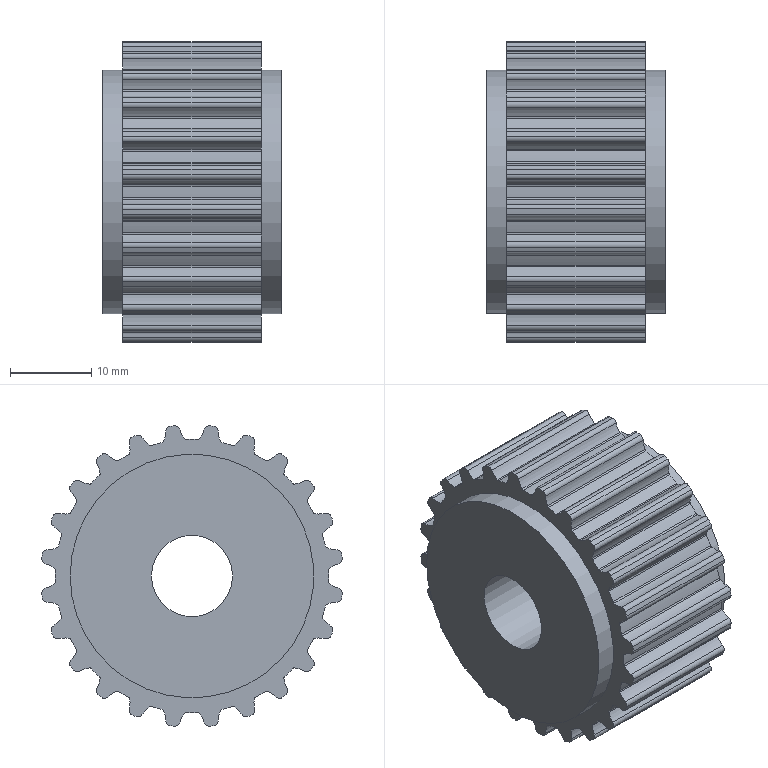Part | NX | features Timing Pulley_5003_015_HTLA24S5M150-E-10 2 | 1 solid | 208 faces | box 22 x 37.006 x 37.006 mm | volume 17570 mm3 | cylinder 199 | plane 5 | cone 4 | commonest cylinder face diameters 0.5 x48 1.1 x48 6.55 x48 33.7 x24 37.24 x24 3.4 x3